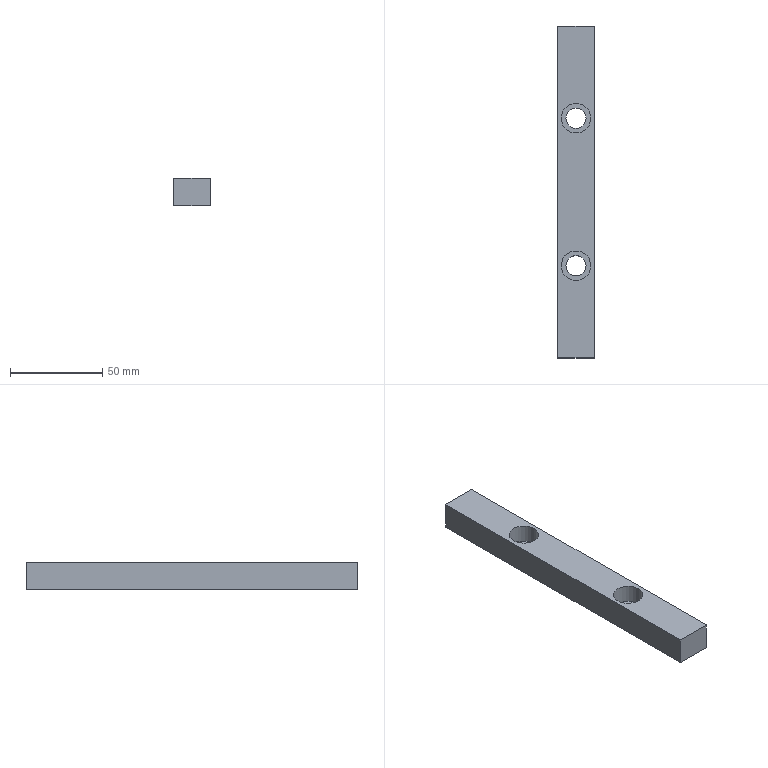Part | NX | features DATUM_CSYS 4, SKETCH 3, CBORE_HOLE 2, EXTRACT_FACE 2, HOLE PACKAGE 2, EXTRUDE 1, Instance Feature 1, Mirror Feature 1 | 1 solid | 12 faces | box 20 x 180 x 15 mm | volume 49028 mm3 | plane 8 | cylinder 4 | commonest cylinder face diameters 11 x2 16 x2
STEP:
#1=CARTESIAN_POINT('',(0.,180.,0.));
#2=VERTEX_POINT('',#1);
#3=CARTESIAN_POINT('',(0.,0.,0.));
#4=VERTEX_POINT('',#3);
#5=CARTESIAN_POINT('',(0.,180.,0.));
#6=DIRECTION('',(0.,-1.,0.));
#7=VECTOR('',#6,1000.);
#8=LINE('',#5,#7);
#9=EDGE_CURVE('',#2,#4,#8,.T.);
#10=ORIENTED_EDGE('',*,*,#9,.T.);
#11=CARTESIAN_POINT('',(0.,0.,15.));
#12=VERTEX_POINT('',#11);
#13=CARTESIAN_POINT('',(0.,0.,15.));
#14=DIRECTION('',(0.,0.,-1.));
#15=VECTOR('',#14,1000.);
#16=LINE('',#13,#15);
#17=EDGE_CURVE('',#12,#4,#16,.T.);
#18=ORIENTED_EDGE('',*,*,#17,.F.);
#19=CARTESIAN_POINT('',(0.,180.,15.));
#20=VERTEX_POINT('',#19);
#21=CARTESIAN_POINT('',(0.,180.,15.));
#22=DIRECTION('',(0.,-1.,0.));
#23=VECTOR('',#22,1000.);
#24=LINE('',#21,#23);
#25=EDGE_CURVE('',#20,#12,#24,.T.);
#26=ORIENTED_EDGE('',*,*,#25,.F.);
#27=CARTESIAN_POINT('',(0.,180.,15.));
#28=DIRECTION('',(0.,0.,-1.));
#29=VECTOR('',#28,1000.);
#30=LINE('',#27,#29);
#31=EDGE_CURVE('',#20,#2,#30,.T.);
#32=ORIENTED_EDGE('',*,*,#31,.T.);
#33=EDGE_LOOP('',(#10,#18,#26,#32));
#34=FACE_BOUND('',#33,.T.);
#35=CARTESIAN_POINT('',(0.,180.,15.));
#36=DIRECTION('',(1.,0.,0.));
#37=DIRECTION('',(0.,1.,0.));
#38=AXIS2_PLACEMENT_3D('',#35,#36,#37);
#39=PLANE('',#38);
#40=ADVANCED_FACE('',(#34),#39,.F.);
#41=CARTESIAN_POINT('',(20.,0.,0.));
#42=VERTEX_POINT('',#41);
#43=CARTESIAN_POINT('',(0.,0.,0.));
#44=DIRECTION('',(1.,0.,0.));
#45=VECTOR('',#44,1000.);
#46=LINE('',#43,#45);
#47=EDGE_CURVE('',#4,#42,#46,.T.);
#48=ORIENTED_EDGE('',*,*,#47,.T.);
#49=CARTESIAN_POINT('',(20.,0.,15.));
#50=VERTEX_POINT('',#49);
#51=CARTESIAN_POINT('',(20.,0.,15.));
#52=DIRECTION('',(0.,0.,-1.));
#53=VECTOR('',#52,1000.);
#54=LINE('',#51,#53);
#55=EDGE_CURVE('',#50,#42,#54,.T.);
#56=ORIENTED_EDGE('',*,*,#55,.F.);
#57=CARTESIAN_POINT('',(0.,0.,15.));
#58=DIRECTION('',(1.,0.,0.));
#59=VECTOR('',#58,1000.);
#60=LINE('',#57,#59);
#61=EDGE_CURVE('',#12,#50,#60,.T.);
#62=ORIENTED_EDGE('',*,*,#61,.F.);
#63=ORIENTED_EDGE('',*,*,#17,.T.);
#64=EDGE_LOOP('',(#48,#56,#62,#63));
#65=FACE_BOUND('',#64,.T.);
#66=CARTESIAN_POINT('',(0.,0.,15.));
#67=DIRECTION('',(0.,1.,0.));
#68=DIRECTION('',(0.,0.,1.));
#69=AXIS2_PLACEMENT_3D('',#66,#67,#68);
#70=PLANE('',#69);
#71=ADVANCED_FACE('',(#65),#70,.F.);
#72=CARTESIAN_POINT('',(20.,180.,0.));
#73=VERTEX_POINT('',#72);
#74=CARTESIAN_POINT('',(20.,0.,0.));
#75=DIRECTION('',(0.,1.,0.));
#76=VECTOR('',#75,1000.);
#77=LINE('',#74,#76);
#78=EDGE_CURVE('',#42,#73,#77,.T.);
#79=ORIENTED_EDGE('',*,*,#78,.T.);
#80=CARTESIAN_POINT('',(20.,180.,15.));
#81=VERTEX_POINT('',#80);
#82=CARTESIAN_POINT('',(20.,180.,15.));
#83=DIRECTION('',(0.,0.,-1.));
#84=VECTOR('',#83,1000.);
#85=LINE('',#82,#84);
#86=EDGE_CURVE('',#81,#73,#85,.T.);
#87=ORIENTED_EDGE('',*,*,#86,.F.);
#88=CARTESIAN_POINT('',(20.,0.,15.));
#89=DIRECTION('',(0.,1.,0.));
#90=VECTOR('',#89,1000.);
#91=LINE('',#88,#90);
#92=EDGE_CURVE('',#50,#81,#91,.T.);
#93=ORIENTED_EDGE('',*,*,#92,.F.);
#94=ORIENTED_EDGE('',*,*,#55,.T.);
#95=EDGE_LOOP('',(#79,#87,#93,#94));
#96=FACE_BOUND('',#95,.T.);
#97=CARTESIAN_POINT('',(20.,0.,15.));
#98=DIRECTION('',(-1.,0.,0.));
#99=DIRECTION('',(0.,-1.,0.));
#100=AXIS2_PLACEMENT_3D('',#97,#98,#99);
#101=PLANE('',#100);
#102=ADVANCED_FACE('',(#96),#101,.F.);
#103=CARTESIAN_POINT('',(20.,180.,0.));
#104=DIRECTION('',(-1.,0.,0.));
#105=VECTOR('',#104,1000.);
#106=LINE('',#103,#105);
#107=EDGE_CURVE('',#73,#2,#106,.T.);
#108=ORIENTED_EDGE('',*,*,#107,.T.);
#109=ORIENTED_EDGE('',*,*,#31,.F.);
#110=CARTESIAN_POINT('',(20.,180.,15.));
#111=DIRECTION('',(-1.,0.,0.));
#112=VECTOR('',#111,1000.);
#113=LINE('',#110,#112);
#114=EDGE_CURVE('',#81,#20,#113,.T.);
#115=ORIENTED_EDGE('',*,*,#114,.F.);
#116=ORIENTED_EDGE('',*,*,#86,.T.);
#117=EDGE_LOOP('',(#108,#109,#115,#116));
#118=FACE_BOUND('',#117,.T.);
#119=CARTESIAN_POINT('',(20.,180.,15.));
#120=DIRECTION('',(0.,-1.,0.));
#121=DIRECTION('',(0.,0.,-1.));
#122=AXIS2_PLACEMENT_3D('',#119,#120,#121);
#123=PLANE('',#122);
#124=ADVANCED_FACE('',(#118),#123,.F.);
#125=CARTESIAN_POINT('',(2.,50.,15.));
#126=VERTEX_POINT('',#125);
#127=CARTESIAN_POINT('',(10.,50.,15.));
#128=DIRECTION('',(0.,0.,-1.));
#129=DIRECTION('',(-1.,0.,0.));
#130=AXIS2_PLACEMENT_3D('',#127,#128,#129);
#131=CIRCLE('',#130,8.);
#132=EDGE_CURVE('',#126,#126,#131,.T.);
#133=ORIENTED_EDGE('',*,*,#132,.T.);
#134=EDGE_LOOP('',(#133));
#135=FACE_BOUND('',#134,.T.);
#136=CARTESIAN_POINT('',(2.,130.,15.));
#137=VERTEX_POINT('',#136);
#138=CARTESIAN_POINT('',(10.,130.,15.));
#139=DIRECTION('',(0.,0.,-1.));
#140=DIRECTION('',(-1.,0.,0.));
#141=AXIS2_PLACEMENT_3D('',#138,#139,#140);
#142=CIRCLE('',#141,8.);
#143=EDGE_CURVE('',#137,#137,#142,.T.);
#144=ORIENTED_EDGE('',*,*,#143,.T.);
#145=EDGE_LOOP('',(#144));
#146=FACE_BOUND('',#145,.T.);
#147=ORIENTED_EDGE('',*,*,#25,.T.);
#148=ORIENTED_EDGE('',*,*,#61,.T.);
#149=ORIENTED_EDGE('',*,*,#92,.T.);
#150=ORIENTED_EDGE('',*,*,#114,.T.);
#151=EDGE_LOOP('',(#147,#148,#149,#150));
#152=FACE_BOUND('',#151,.T.);
#153=CARTESIAN_POINT('',(0.,0.,15.));
#154=DIRECTION('',(0.,0.,1.));
#155=DIRECTION('',(1.,0.,0.));
#156=AXIS2_PLACEMENT_3D('',#153,#154,#155);
#157=PLANE('',#156);
#158=ADVANCED_FACE('',(#135,#146,#152),#157,.T.);
#159=CARTESIAN_POINT('',(15.5,50.,0.));
#160=VERTEX_POINT('',#159);
#161=CARTESIAN_POINT('',(10.,50.,0.));
#162=DIRECTION('',(0.,0.,1.));
#163=DIRECTION('',(1.,0.,0.));
#164=AXIS2_PLACEMENT_3D('',#161,#162,#163);
#165=CIRCLE('',#164,5.5);
#166=EDGE_CURVE('',#160,#160,#165,.T.);
#167=ORIENTED_EDGE('',*,*,#166,.T.);
#168=EDGE_LOOP('',(#167));
#169=FACE_BOUND('',#168,.T.);
#170=CARTESIAN_POINT('',(15.5,130.,0.));
#171=VERTEX_POINT('',#170);
#172=CARTESIAN_POINT('',(10.,130.,0.));
#173=DIRECTION('',(0.,0.,1.));
#174=DIRECTION('',(1.,0.,0.));
#175=AXIS2_PLACEMENT_3D('',#172,#173,#174);
#176=CIRCLE('',#175,5.5);
#177=EDGE_CURVE('',#171,#171,#176,.T.);
#178=ORIENTED_EDGE('',*,*,#177,.T.);
#179=EDGE_LOOP('',(#178));
#180=FACE_BOUND('',#179,.T.);
#181=ORIENTED_EDGE('',*,*,#9,.F.);
#182=ORIENTED_EDGE('',*,*,#107,.F.);
#183=ORIENTED_EDGE('',*,*,#78,.F.);
#184=ORIENTED_EDGE('',*,*,#47,.F.);
#185=EDGE_LOOP('',(#181,#182,#183,#184));
#186=FACE_BOUND('',#185,.T.);
#187=CARTESIAN_POINT('',(0.,0.,0.));
#188=DIRECTION('',(0.,0.,1.));
#189=DIRECTION('',(1.,0.,0.));
#190=AXIS2_PLACEMENT_3D('',#187,#188,#189);
#191=PLANE('',#190);
#192=ADVANCED_FACE('',(#169,#180,#186),#191,.F.);
#193=CARTESIAN_POINT('',(4.5,130.,5.));
#194=VERTEX_POINT('',#193);
#195=CARTESIAN_POINT('',(10.,130.,5.));
#196=DIRECTION('',(0.,0.,-1.));
#197=DIRECTION('',(-1.,0.,0.));
#198=AXIS2_PLACEMENT_3D('',#195,#196,#197);
#199=CIRCLE('',#198,5.5);
#200=EDGE_CURVE('',#194,#194,#199,.F.);
#201=ORIENTED_EDGE('',*,*,#200,.T.);
#202=EDGE_LOOP('',(#201));
#203=FACE_BOUND('',#202,.T.);
#204=ORIENTED_EDGE('',*,*,#177,.F.);
#205=EDGE_LOOP('',(#204));
#206=FACE_BOUND('',#205,.T.);
#207=CARTESIAN_POINT('',(10.,130.,-485.));
#208=DIRECTION('',(0.,0.,-1.));
#209=DIRECTION('',(-1.,0.,0.));
#210=AXIS2_PLACEMENT_3D('',#207,#208,#209);
#211=CYLINDRICAL_SURFACE('',#210,5.5);
#212=ADVANCED_FACE('',(#203,#206),#211,.F.);
#213=ORIENTED_EDGE('',*,*,#200,.F.);
#214=EDGE_LOOP('',(#213));
#215=FACE_BOUND('',#214,.T.);
#216=CARTESIAN_POINT('',(2.,130.,5.));
#217=VERTEX_POINT('',#216);
#218=CARTESIAN_POINT('',(10.,130.,5.));
#219=DIRECTION('',(0.,0.,-1.));
#220=DIRECTION('',(-1.,0.,0.));
#221=AXIS2_PLACEMENT_3D('',#218,#219,#220);
#222=CIRCLE('',#221,8.);
#223=EDGE_CURVE('',#217,#217,#222,.F.);
#224=ORIENTED_EDGE('',*,*,#223,.T.);
#225=EDGE_LOOP('',(#224));
#226=FACE_BOUND('',#225,.T.);
#227=CARTESIAN_POINT('',(10.,130.,5.));
#228=DIRECTION('',(0.,0.,-1.));
#229=DIRECTION('',(-1.,0.,0.));
#230=AXIS2_PLACEMENT_3D('',#227,#228,#229);
#231=PLANE('',#230);
#232=ADVANCED_FACE('',(#215,#226),#231,.F.);
#233=ORIENTED_EDGE('',*,*,#223,.F.);
#234=EDGE_LOOP('',(#233));
#235=FACE_BOUND('',#234,.T.);
#236=ORIENTED_EDGE('',*,*,#143,.F.);
#237=EDGE_LOOP('',(#236));
#238=FACE_BOUND('',#237,.T.);
#239=CARTESIAN_POINT('',(10.,130.,15.));
#240=DIRECTION('',(0.,0.,-1.));
#241=DIRECTION('',(-1.,0.,0.));
#242=AXIS2_PLACEMENT_3D('',#239,#240,#241);
#243=CYLINDRICAL_SURFACE('',#242,8.);
#244=ADVANCED_FACE('',(#235,#238),#243,.F.);
#245=CARTESIAN_POINT('',(4.5,50.,5.));
#246=VERTEX_POINT('',#245);
#247=CARTESIAN_POINT('',(10.,50.,5.));
#248=DIRECTION('',(0.,0.,-1.));
#249=DIRECTION('',(-1.,0.,0.));
#250=AXIS2_PLACEMENT_3D('',#247,#248,#249);
#251=CIRCLE('',#250,5.5);
#252=EDGE_CURVE('',#246,#246,#251,.T.);
#253=ORIENTED_EDGE('',*,*,#252,.F.);
#254=EDGE_LOOP('',(#253));
#255=FACE_BOUND('',#254,.T.);
#256=ORIENTED_EDGE('',*,*,#166,.F.);
#257=EDGE_LOOP('',(#256));
#258=FACE_BOUND('',#257,.T.);
#259=CARTESIAN_POINT('',(10.,50.,-485.));
#260=DIRECTION('',(0.,0.,-1.));
#261=DIRECTION('',(-1.,0.,0.));
#262=AXIS2_PLACEMENT_3D('',#259,#260,#261);
#263=CYLINDRICAL_SURFACE('',#262,5.5);
#264=ADVANCED_FACE('',(#255,#258),#263,.F.);
#265=ORIENTED_EDGE('',*,*,#252,.T.);
#266=EDGE_LOOP('',(#265));
#267=FACE_BOUND('',#266,.T.);
#268=CARTESIAN_POINT('',(2.,50.,5.));
#269=VERTEX_POINT('',#268);
#270=CARTESIAN_POINT('',(10.,50.,5.));
#271=DIRECTION('',(0.,0.,-1.));
#272=DIRECTION('',(-1.,0.,0.));
#273=AXIS2_PLACEMENT_3D('',#270,#271,#272);
#274=CIRCLE('',#273,8.);
#275=EDGE_CURVE('',#269,#269,#274,.T.);
#276=ORIENTED_EDGE('',*,*,#275,.F.);
#277=EDGE_LOOP('',(#276));
#278=FACE_BOUND('',#277,.T.);
#279=CARTESIAN_POINT('',(10.,50.,5.));
#280=DIRECTION('',(0.,0.,-1.));
#281=DIRECTION('',(-1.,0.,0.));
#282=AXIS2_PLACEMENT_3D('',#279,#280,#281);
#283=PLANE('',#282);
#284=ADVANCED_FACE('',(#267,#278),#283,.F.);
#285=ORIENTED_EDGE('',*,*,#275,.T.);
#286=EDGE_LOOP('',(#285));
#287=FACE_BOUND('',#286,.T.);
#288=ORIENTED_EDGE('',*,*,#132,.F.);
#289=EDGE_LOOP('',(#288));
#290=FACE_BOUND('',#289,.T.);
#291=CARTESIAN_POINT('',(10.,50.,15.));
#292=DIRECTION('',(0.,0.,-1.));
#293=DIRECTION('',(-1.,0.,0.));
#294=AXIS2_PLACEMENT_3D('',#291,#292,#293);
#295=CYLINDRICAL_SURFACE('',#294,8.);
#296=ADVANCED_FACE('',(#287,#290),#295,.F.);
#297=CLOSED_SHELL('',(#40,#71,#102,#124,#158,#192,#212,#232,#244,#264,#284,#296));
#298=MANIFOLD_SOLID_BREP('',#297);
#299=(LENGTH_UNIT()NAMED_UNIT(*)SI_UNIT(.MILLI.,.METRE.));
#300=UNCERTAINTY_MEASURE_WITH_UNIT(LENGTH_MEASURE(0.00001),#299,'','');
#301=(NAMED_UNIT(*)PLANE_ANGLE_UNIT()SI_UNIT($,.RADIAN.));
#302=(NAMED_UNIT(*)SI_UNIT($,.STERADIAN.)SOLID_ANGLE_UNIT());
#303=(GEOMETRIC_REPRESENTATION_CONTEXT(3)GLOBAL_UNCERTAINTY_ASSIGNED_CONTEXT((#300))GLOBAL_UNIT_ASSIGNED_CONTEXT((#299,#301,#302))REPRESENTATION_CONTEXT('',''));
#304=ADVANCED_BREP_SHAPE_REPRESENTATION('',(#298),#303);